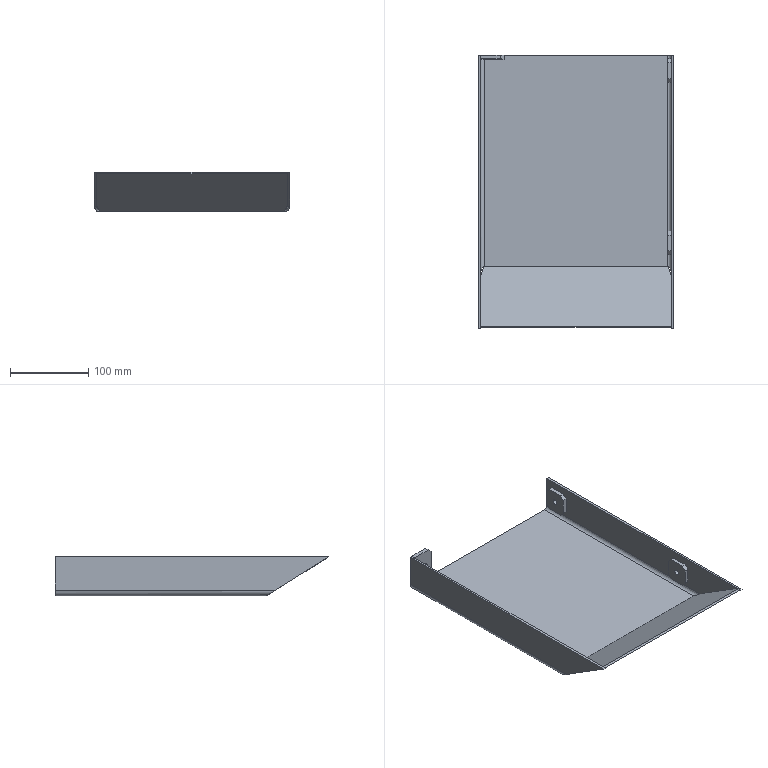Part | SolidWorks | features ICE 5, Chamfer 3, EdgeFlange 1, FlatPattern 1, HoleWzd 1, SMBaseFlange 1, SheetMetal 1 | 5 solids | 75 faces | box 250 x 350 x 50.917 mm | volume 357270 mm3 | plane 56 | cylinder 14 | spline 5 | commonest cylinder face diameters 6.8 x8 9 x4 15 x2